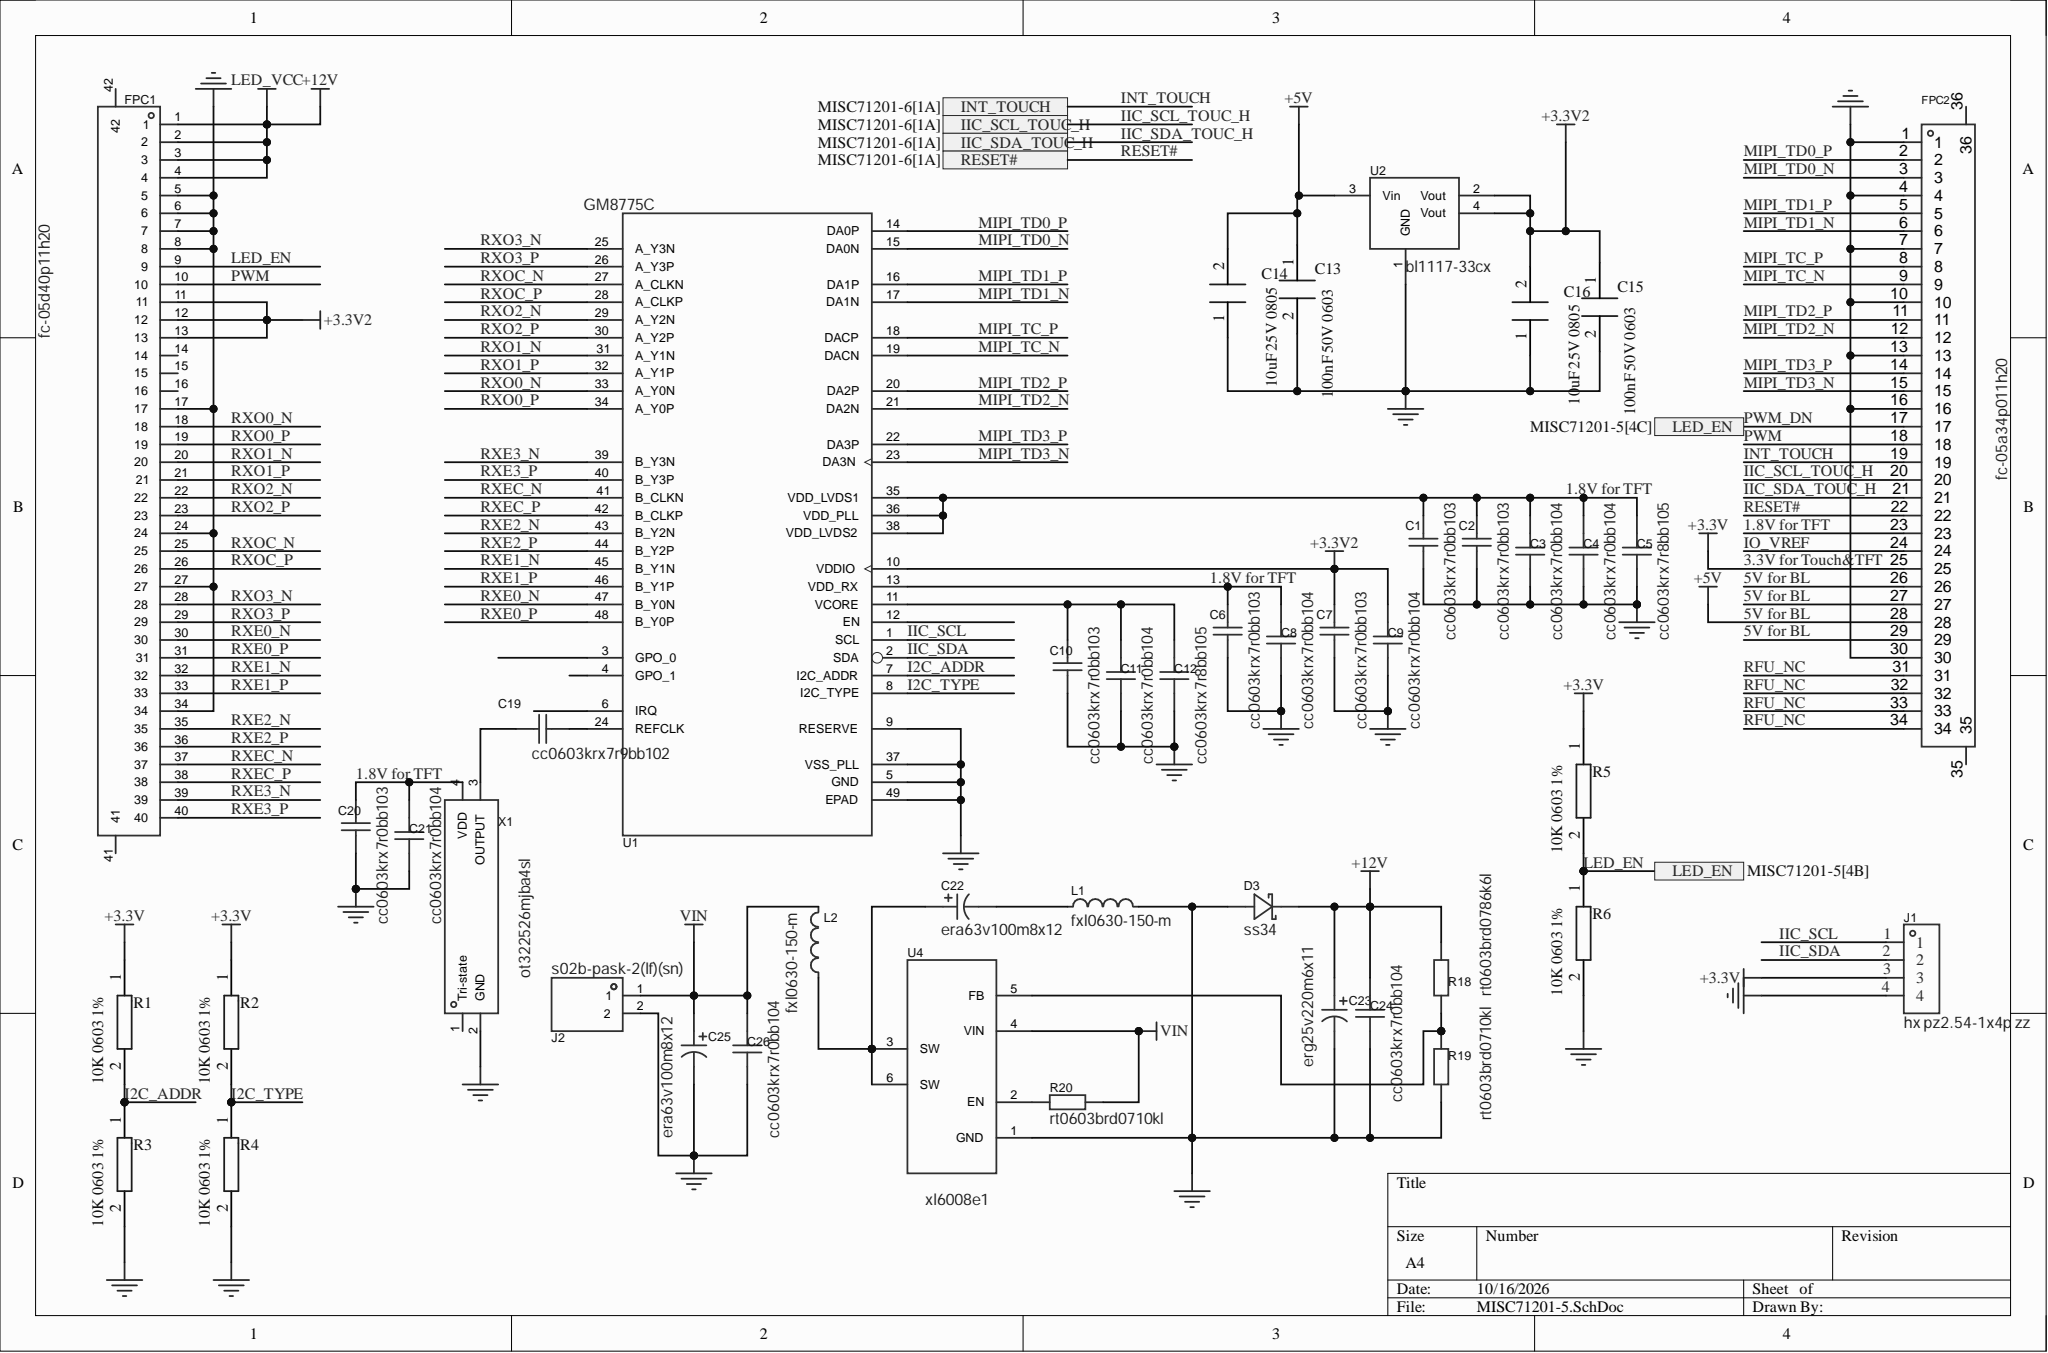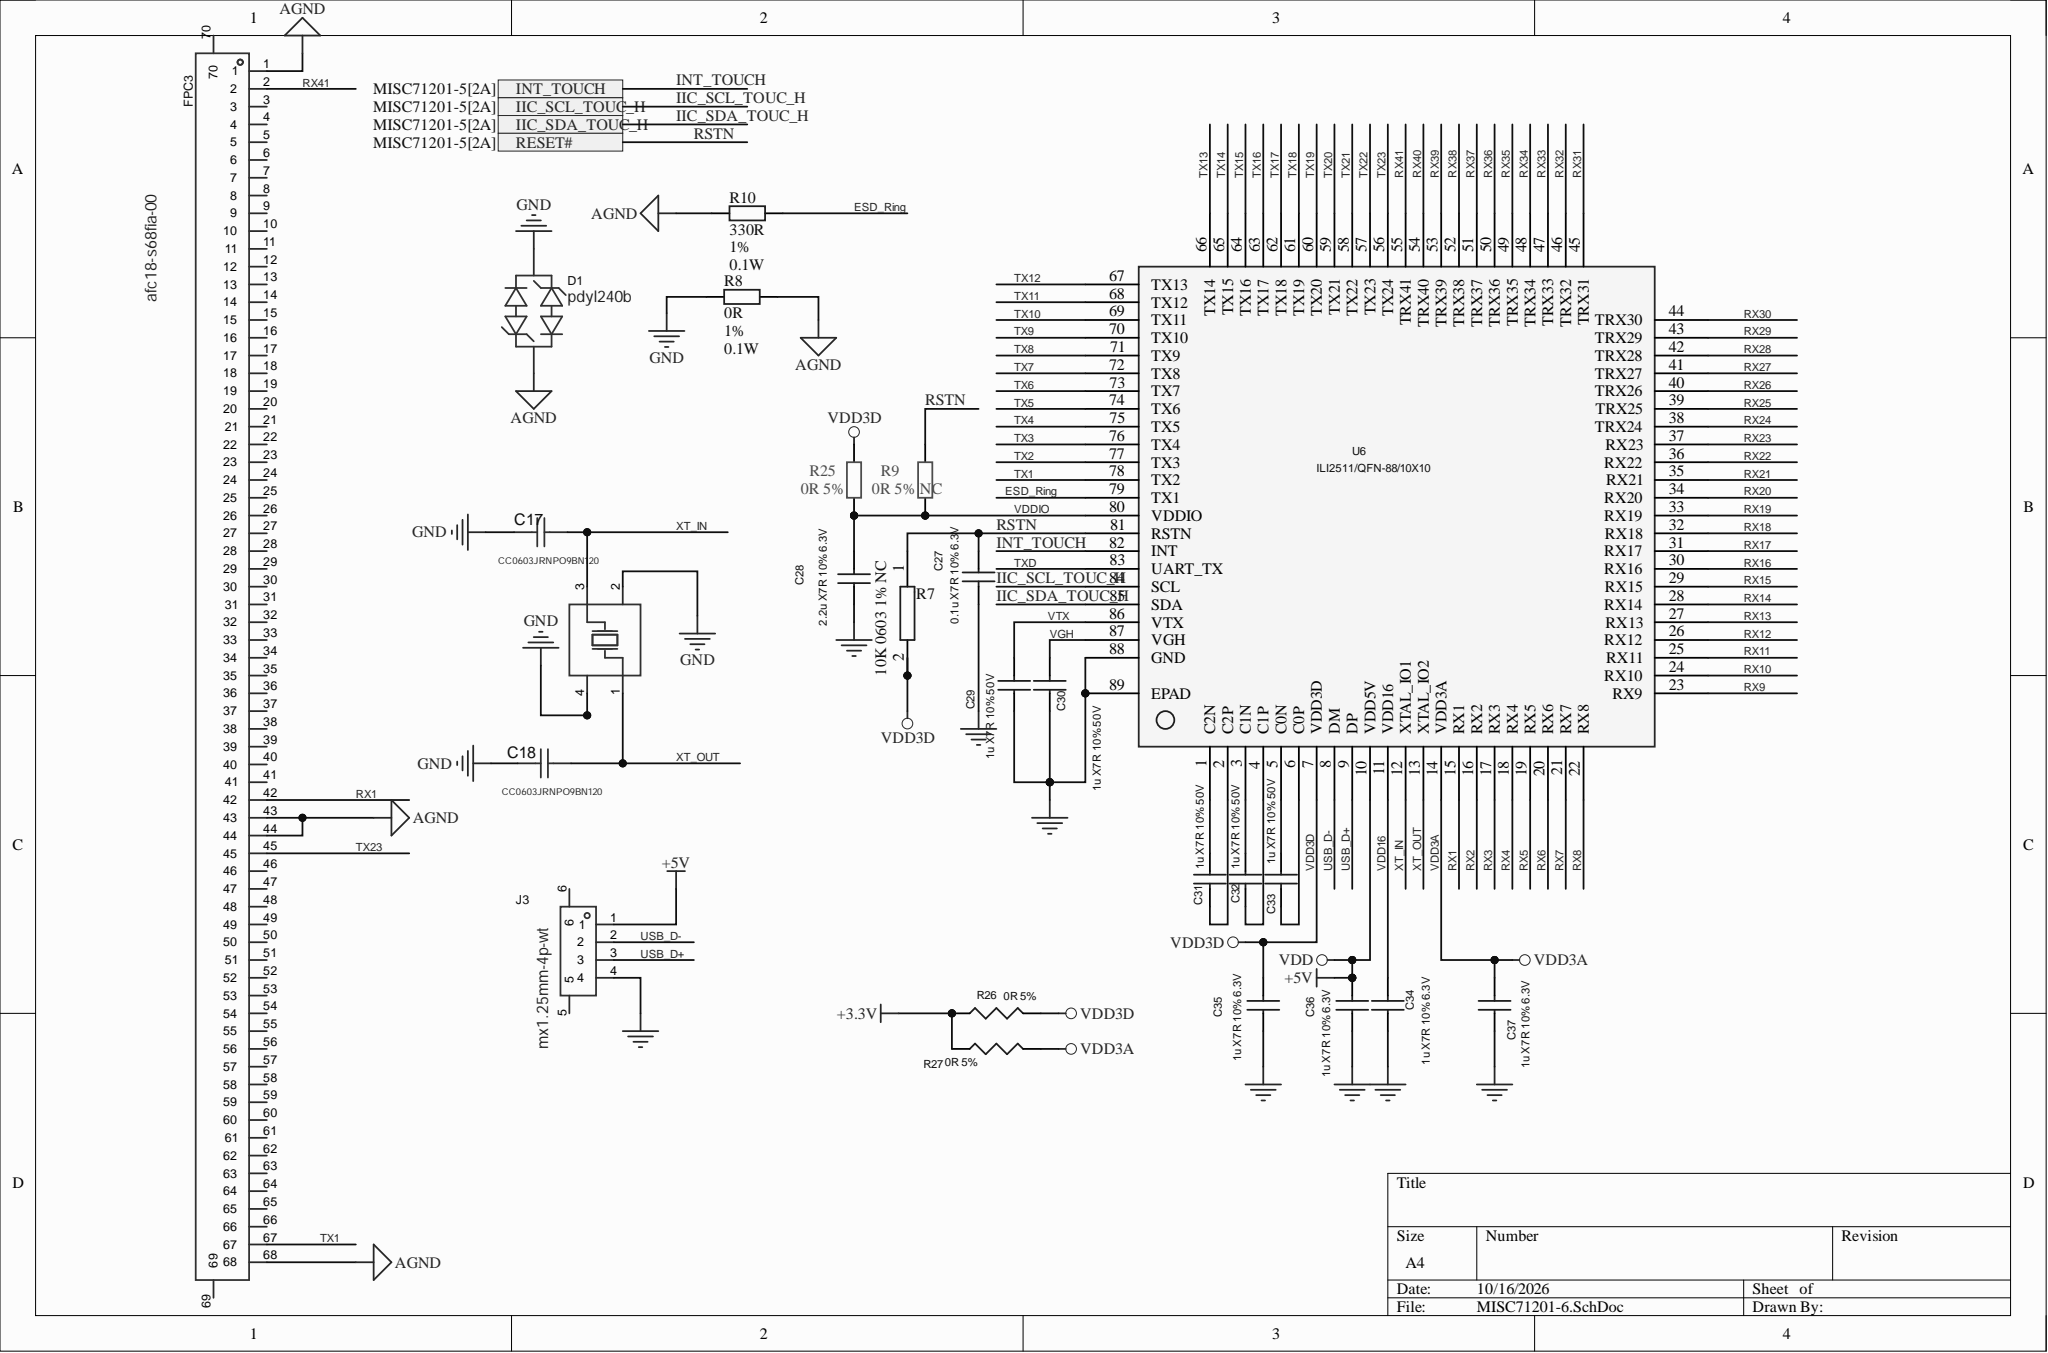Circuit board | Altium Designer | 69 parts | 77 nets
Bill of materials:
Comment,Description,Designator,Footprint,LibRef,Quantity
"cc0603krx7r0bb103","Capacitance:10nF;Tolerance:±10%;Rated voltage:100V;Temp. coefficient:X7R;","C1, C2, C6, C7, C10, C20","C0603","cc0603krx7r0bb103","6"
"cc0603krx7r0bb104","Capacitance:100nF;Tolerance:±10%;Rated voltage:100V;Temp. coefficient:X7R;","C3, C4, C8, C9, C11, C21, C24, C26","C0603","cc0603krx7r0bb104","8"
"cc0603krx7r8bb105","Capacitance:1uF;Tolerance:±10%;Rated voltage:25V;Temp. coefficient:X7R;","C5, C12","C0603","cc0603krx7r8bb105","2"
"100nF 50V 0603","","C13, C15","CAP C0603","CAPACITOR CER","2"
"10uF 25V 0805","","C14, C16","CAP C0805","CAPACITOR CER","2"
"CC0603JRNPO9BN120","12PF","C17, C18","CAP C0603","CC0603JRNPO9BN120","2"
"cc0603krx7r9bb102","Capacitance:1nF;Tolerance:±10%;Rated voltage:50V;Material (temp. coefficient):X7R;","C19","C0603","cc0603krx7r9bb102","1"
"era63v100m8x12","Capacitance:100uF;Tolerance:±20%;Rated voltage:63V;Ripple current:215mA@120Hz;Equivalent series resistance (ESR):-;","C22, C25","CAP-TH_BD8.0-P3.50-D0.8-FD","era63v100m8x12","2"
"erg25v220m6x11","Capacitance:220uF;Tolerance:±20%;Rated voltage:25V;Ripple current:510mA@100kHz;Equivalent series resistance (ESR):130mO@100kHz;","C23","CAP-TH_BD6.3-P2.50-D0.5-FD","erg25v220m6x11","1"
"0.1u X7R 10% 6.3V","SMD capacitor","C27","C0603","C0402_1u_6.3V_X5R","1"
"2.2u X7R 10% 6.3V","SMD capacitor","C28","C0603","C0402_2.2u_6.3V_X5R","1"
"1u X7R 10% 50V","SMD capacitor","C29, C30, C31, C32, C33","C0603","C0603_1u_50V_X7R","5"
"1u X7R 10% 6.3V","SMD capacitor","C34, C35, C36, C37","C0603","C0402_2.2u_6.3V_X5R","4"
"pdyl240b","Reverse standoff voltage (Vrwm):24V;Clamping voltage:60V;Peak pulse power (Ppp):350W@8/20us;Breakdown voltage (VBR):26.7V;","D1","SOD-323_L1.8-W1.3-LS2.5-RD","pdyl240b_c5187140","1"
"ss34","Diode configuration:Single;Forward voltage (Vf):550mV@3A;DC reverse voltage (Vr):40V;Rectified current:3A;","D3","SMA_L4.3-W2.6-LS5.0-RD","ss34_c7420365","1"
"fc-05d40p11h20","Locking:Slide;Contact type:Bottom;Contacts:40P;Pitch:0.5mm;Mounting:Horizontal SMT;Operating temperature:-25℃~+85℃;","FPC1","FPC-SMD_40P-P0.50_FC-05D40P11H20","fc-05d40p11h20","1"
"fc-05a34p011h20","Locking:Flip;Contact type:Bottom;Contacts:34P;Pitch:0.5mm;Mounting:Horizontal SMT;Operating temperature:-40℃~+85℃;","FPC2","FPC-SMD_FC-05A34P011H20","fc-05a34p011h20","1"
"afc18-s68fia-00","Locking:Flip;Contact type:Bottom;Contacts:68P;Pitch:0.5mm;Mounting:Horizontal SMT;Operating temperature:-25℃~+85℃;","FPC3","CONN-SMD_AFC18-S68FIA-00","afc18-s68fia-00","1"
"hx pz2.54-1x4p zz","Pin structure:1x4P;Pitch:2.54mm;Row pitch:-;Round/square pin:Square;Mounting:THT;Rows:Single;Total pins:4P;Rated current:3A;Rated voltage:1kV;Mating pin length:6mm;Insulator height:2.5mm;Tail length:3mm;Contact material:Brass;Contact plating:Gold;Operating temperature:-40℃~+105℃;Color:Black;","J1","HDR-TH_4P-P2.54-V-M","hx pz2.54-1x4p zz","1"
"s02b-pask-2(lf)(sn)","Pin structure:1x2P;Pitch:2mm;Mounting:Right-angle THT;Series:PA;Total pins:2P;Rows:1;Pins per row:2;Row pitch:-;Rated current:3A;Contact material:Copper alloy;Contact plating:Tin;Operating temperature:-25℃~+85℃;","J2","CONN-TH_S02B-PASK-2-LF-SN","s02b-pask-2(lf)(sn)","1"
"mx1.25mm-4p-wt","Pin structure:1x4P;Pitch:1.25mm;Mounting:Horizontal SMT;Series:PicoBlade(MX 1.25);Total pins:4P;Rows:1;Pins per row:4;Rated current:1A;Contact material:Brass;Contact plating:Tin;Operating temperature:-25℃~+85℃;","J3","CONN-SMD_MX1.25MM-4P-WT","mx1.25mm-4p-wt","1"
"fxl0630-150-m","SMD, 7x6.6x2.8mm   alloy inductor, molded inductor, high current","L1, L2","IND-SMD_L7.0-W6.6_FXL0630","fxl0630-150-m","2"
"10K 0603 1%","","R1, R2, R3, R4, R5, R6","RES R0603","Resistor","6"
"10K 0603 1% NC","","R7","RES R0603","Resistor","1"
"0R 0603","","R8, R10","RES R0603","Res2","2"
"0R 5% NC","SMD resistor","R9","R0603","Res2","1"
"rt0603brd0786k6l","Resistor type:Thin film;Resistance:86.6kO;Tolerance:±0.1%;Power:100mW;Temp. coefficient:±25ppm/?;","R18","R0603","rt0603brd0786k6l","1"
"rt0603brd0710kl","Resistor type:Thin film;Resistance:10kO;Tolerance:±0.1%;Power:100mW;Operating voltage:75V;Temp. coefficient:±25ppm/?;","R19, R20","R0603","rt0603brd0710kl","2"
"0R 5%","SMD resistor","R25","R0603","Res2","1"
"0R 5%","SMD resistor","R26, R27","R0402","R0402_0R_+-5%_Dup2","2"
"GM8775C","CPU core:ARM Cortex-M4;CPU max frequency:100MHz;CPU bits:32 Bit;","U1","UFQFPN-48_L7.0-W7.0-P0.50-BL-EP","stm32f411ceu6","1"
"bl1117-33cx","Output polarity:Positive;Operating voltage:12V;Output voltage:3.3V;Output current:1A;PSRR:60dB@(120Hz);Output type:Fixed;","U2","SOT-223_L6.5-W3.5-P2.30-LS7.0-BR","bl1117-33cx","1"
"xl6008e1","Function:Buck-boost;Operating voltage:3.6V~32V;Output voltage:-;Output current:3A;Output type:Adjustable;","U4","TO-252-5_L6.6-W5.8-P1.27-TL","xl6008e1","1"
"ILI2511/QFN-88/10X10","ILITEK IC","U6","ILI2511/QFN-88/10X10","ILI2511/QFN-88/10X10_0.4_0.9","1"
"ot322526mjba4sl","Frequency:26MHz;Frequency tolerance (room temp.):±10ppm;Output:CMOS;Operating voltage:1.8V~3.3V;Frequency stability:±20ppm;","X1","OSC-SMD_4P-L3.2-W2.5-BL","ot322526mjba4sl","1"
"x322512msb4si","Crystal type:SMD crystal;Frequency:12MHz;Frequency tolerance (room temp.):±10ppm;Load capacitance:20pF;Frequency stability:±20ppm;","X2","CRYSTAL-SMD_4P-L3.2-W2.5-BL","x322512msb4si","1"
Netlist (Protel format):
[
C1
C0603
cc0603krx7r0bb103



]
[
C2
C0603
cc0603krx7r0bb103



]
[
C3
C0603
cc0603krx7r0bb104



]
[
C4
C0603
cc0603krx7r0bb104



]
[
C5
C0603
cc0603krx7r8bb105



]
[
C6
C0603
cc0603krx7r0bb103



]
[
C7
C0603
cc0603krx7r0bb103



]
[
C8
C0603
cc0603krx7r0bb104



]
[
C9
C0603
cc0603krx7r0bb104



]
[
C10
C0603
cc0603krx7r0bb103



]
[
C11
C0603
cc0603krx7r0bb104



]
[
C12
C0603
cc0603krx7r8bb105



]
[
C13
CAP C0603
100nF 50V 0603



]
[
C14
CAP C0805
10uF 25V 0805



]
[
C15
CAP C0603
100nF 50V 0603



]
[
C16
CAP C0805
10uF 25V 0805



]
[
C17
CAP C0603
CC0603JRNPO9BN120



]
[
C18
CAP C0603
CC0603JRNPO9BN120



]
[
C19
C0603
cc0603krx7r9bb102



]
[
C20
C0603
cc0603krx7r0bb103



]
[
C21
C0603
cc0603krx7r0bb104



]
[
C22
CAP-TH_BD8.0-P3.50-D0.8-FD
era63v100m8x12



]
[
C23
CAP-TH_BD6.3-P2.50-D0.5-FD
erg25v220m6x11



]
[
C24
C0603
cc0603krx7r0bb104



]
[
C25
CAP-TH_BD8.0-P3.50-D0.8-FD
era63v100m8x12



]
[
C26
C0603
cc0603krx7r0bb104



]
[
C27
C0603
0.1u X7R 10% 6.3V



]
[
C28
C0603
2.2u X7R 10% 6.3V



]
[
C29
C0603
1u X7R 10% 50V



]
[
C30
C0603
1u X7R 10% 50V



]
[
C31
C0603
1u X7R 10% 50V



]
[
C32
C0603
1u X7R 10% 50V



]
[
C33
C0603
1u X7R 10% 50V



]
[
C34
C0603
1u X7R 10% 6.3V



]
[
C35
C0603
1u X7R 10% 6.3V



]
[
C36
C0603
1u X7R 10% 6.3V



]
[
C37
C0603
1u X7R 10% 6.3V



]
[
D1
SOD-323_L1.8-W1.3-LS2.5-RD
pdyl240b



]
[
D3
SMA_L4.3-W2.6-LS5.0-RD
ss34



]
[
FPC1
FPC-SMD_40P-P0.50_FC-05D40P11H20
fc-05d40p11h20



]
[
FPC2
FPC-SMD_FC-05A34P011H20
fc-05a34p011h20



]
[
FPC3
CONN-SMD_AFC18-S68FIA-00
afc18-s68fia-00



]
[
J1
HDR-TH_4P-P2.54-V-M
hx pz2.54-1x4p zz



]
[
J2
CONN-TH_S02B-PASK-2-LF-SN
s02b-pask-2(lf)(sn)



]
[
J3
CONN-SMD_MX1.25MM-4P-WT
mx1.25mm-4p-wt



]
[
L1
IND-SMD_L7.0-W6.6_FXL0630
fxl0630-150-m



]
[
L2
IND-SMD_L7.0-W6.6_FXL0630
fxl0630-150-m



]
[
R1
RES R0603
10K 0603 1%



]
[
R2
RES R0603
10K 0603 1%



]
[
R3
RES R0603
10K 0603 1%



]
[
R4
RES R0603
10K 0603 1%



]
[
R5
RES R0603
10K 0603 1%



]
[
R6
RES R0603
10K 0603 1%



]
[
R7
RES R0603
10K 0603 1% NC



]
[
R8
RES R0603
0R 0603



]
[
R9
R0603
0R 5% NC



]
[
R10
RES R0603
0R 0603



]
[
R18
R0603
rt0603brd0786k6l



]
[
R19
R0603
rt0603brd0710kl



]
[
R20
R0603
rt0603brd0710kl



]
[
R25
R0603
0R 5%



]
[
R26
R0402
0R 5%



]
[
R27
R0402
0R 5%



]
[
U1
UFQFPN-48_L7.0-W7.0-P0.50-BL-EP
GM8775C



]
[
U2
SOT-223_L6.5-W3.5-P2.30-LS7.0-BR
bl1117-33cx



]
[
U4
TO-252-5_L6.6-W5.8-P1.27-TL
xl6008e1



]
[
U6
ILI2511/QFN-88/10X10
ILI2511/QFN-88/10X10



]
[
X1
OSC-SMD_4P-L3.2-W2.5-BL
ot322526mjba4sl



]
[
X2
CRYSTAL-SMD_4P-L3.2-W2.5-BL
x322512msb4si



]
(
XT_OUT
C18-2
U6-13
X2-1
)
(
XT_IN
C17-2
U6-12
X2-3
)
(
VTX
C29-2
U6-86
)
(
VIN
C25-1
C26-2
J2-1
L2-2
R20-2
U4-4
)
(
VGH
C30-2
U6-87
)
(
VDDIO
C28-2
R9-1
R25-1
U6-80
)
(
VDD16
C34-2
U6-11
)
(
VDD3D
C35-2
R7-2
R25-2
R26-2
U6-7
)
(
VDD3A
C37-2
R27-2
U6-14
)
(
USB_D-
J3-2
U6-8
)
(
USB_D+
J3-3
U6-9
)
(
TX23
FPC3-45
U6-56
)
(
TX1
FPC3-67
U6-78
)
(
RXOC_P
FPC1-26
U1-28
)
(
RXOC_N
FPC1-25
U1-27
)
(
RXO3_P
FPC1-29
U1-26
)
(
RXO3_N
FPC1-28
U1-25
)
(
RXO2_P
FPC1-23
U1-30
)
(
RXO2_N
FPC1-22
U1-29
)
(
RXO1_P
FPC1-21
U1-32
)
(
RXO1_N
FPC1-20
U1-31
)
(
RXO0_P
FPC1-19
U1-34
)
(
RXO0_N
FPC1-18
U1-33
)
(
RXEC_P
FPC1-38
U1-42
)
(
RXEC_N
FPC1-37
U1-41
)
(
RXE3_P
FPC1-40
U1-40
)
(
RXE3_N
FPC1-39
U1-39
)
(
RXE2_P
FPC1-36
U1-44
)
(
RXE2_N
FPC1-35
U1-43
)
(
RXE1_P
FPC1-33
U1-46
)
(
RXE1_N
FPC1-32
U1-45
)
(
RXE0_P
FPC1-31
U1-48
)
(
RXE0_N
FPC1-30
U1-47
)
(
RX41
FPC3-2
U6-55
)
(
RX1
FPC3-42
U6-15
)
(
RFU_NC
FPC2-31
FPC2-32
FPC2-33
FPC2-34
)
(
RESET#
C27-1
FPC2-22
R7-1
R9-2
U6-81
)
(
PWM
FPC1-10
FPC2-18
)
(
NetR20_1
R20-1
U4-2
)
(
NetR18_1
R18-1
R19-1
U4-5
)
(
NetC33_2
C33-2
U6-6
)
(
NetC33_1
C33-1
U6-5
)
(
NetC32_2
C32-2
U6-4
)
(
NetC32_1
C32-1
U6-3
)
(
NetC31_2
C31-2
U6-2
)
(
NetC31_1
C31-1
U6-1
)
(
NetC22_2
C22-2
L1-1
)
(
NetC22_1
C22-1
L2-1
U4-3
U4-6
)
(
NetC19_2
C19-2
X1-3
)
(
NetC19_1
C19-1
U1-24
)
(
NetC10_2
C10-2
C11-2
C12-1
U1-11
)
(
MIPI_TD3_P
FPC2-14
U1-22
)
(
MIPI_TD3_N
FPC2-15
U1-23
)
(
MIPI_TD2_P
FPC2-11
U1-20
)
(
MIPI_TD2_N
FPC2-12
U1-21
)
(
MIPI_TD1_P
FPC2-5
U1-16
)
(
MIPI_TD1_N
FPC2-6
U1-17
)
(
MIPI_TD0_P
FPC2-2
U1-14
)
(
MIPI_TD0_N
FPC2-3
U1-15
)
(
MIPI_TC_P
FPC2-8
U1-18
)
(
MIPI_TC_N
FPC2-9
U1-19
)
(
LED_EN
FPC1-9
FPC2-17
R5-2
R6-1
)
(
INT_TOUCH
FPC2-19
U6-82
)
(
IIC_SDA_TOUC_H
FPC2-21
U6-85
)
(
IIC_SDA
J1-2
U1-2
)
(
IIC_SCL_TOUC_H
FPC2-20
U6-84
)
(
IIC_SCL
J1-1
U1-1
)
(
I2C_TYPE
R2-2
R4-1
U1-8
)
(
I2C_ADDR
R1-2
R3-1
U1-7
)
(
GND
C1-1
C2-1
C3-1
C4-1
C5-2
C6-1
C7-1
C8-1
C9-1
C10-1
C11-1
C12-2
C13-2
C14-1
C15-2
C16-1
C17-1
C18-1
C20-1
C21-1
C23-2
C24-1
C25-2
C26-1
C27-2
C28-1
C29-1
C30-1
C34-1
C35-1
C36-1
C37-1
D1-1
D3-2
FPC1-5
FPC1-6
FPC1-7
FPC1-8
FPC1-17
FPC1-24
FPC1-27
FPC1-34
FPC2-1
FPC2-4
FPC2-7
FPC2-10
FPC2-13
FPC2-16
FPC2-30
J1-4
J2-2
J3-4
L1-2
R3-2
R4-2
R6-2
R8-1
R19-2
U1-5
U1-9
U1-37
U1-49
U2-1
U4-1
U6-88
U6-89
X1-2
X2-2
X2-4
)
(
ESD_Ring
R10-2
U6-79
)
(
AGND
D1-2
FPC3-1
FPC3-43
FPC3-44
FPC3-68
R8-2
R10-1
)
(
+12V
C23-1
C24-2
D3-1
FPC1-1
FPC1-2
FPC1-3
FPC1-4
R18-2
)
(
+3.3V2
C7-2
C9-2
C15-1
C16-2
FPC1-11
FPC1-12
FPC1-13
U1-10
U2-2
U2-4
)
(
5V for BL
C13-1
C14-2
C36-2
FPC2-26
FPC2-27
FPC2-28
FPC2-29
J3-1
U2-3
U6-10
)
(
3.3V for Touch&TFT
FPC2-25
J1-3
R1-1
R2-1
R5-1
R26-1
R27-1
)
(
1.8V for TFT
C1-2
C2-2
C3-2
C4-2
C5-1
C6-2
C8-2
C20-2
C21-2
FPC2-23
U1-13
U1-35
U1-36
U1-38
X1-4
)